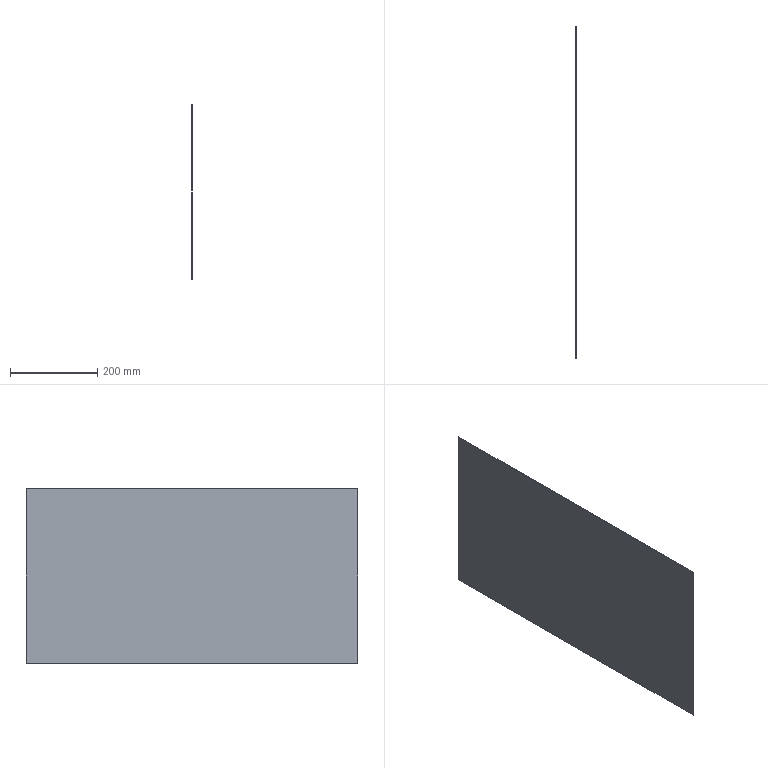Part | STEP file | Guide wheel mechanism revised.sldasm-Part-168 | 1 solid | 6 faces | box 1.2 x 760 x 400 mm | volume 364800 mm3 | plane 6
STEP:
#1=CARTESIAN_POINT('',(-360.,760.,200.));
#2=VERTEX_POINT('',#1);
#3=CARTESIAN_POINT('',(-360.,0.,200.));
#4=VERTEX_POINT('',#3);
#5=CARTESIAN_POINT('',(-360.,760.,200.));
#6=DIRECTION('',(0.,-1.,0.));
#7=VECTOR('',#6,1000.);
#8=LINE('',#5,#7);
#9=EDGE_CURVE('',#2,#4,#8,.T.);
#10=ORIENTED_EDGE('',*,*,#9,.F.);
#11=CARTESIAN_POINT('',(-361.2,760.,200.));
#12=VERTEX_POINT('',#11);
#13=CARTESIAN_POINT('',(-361.2,760.,200.));
#14=DIRECTION('',(1.,0.,0.));
#15=VECTOR('',#14,1000.);
#16=LINE('',#13,#15);
#17=EDGE_CURVE('',#12,#2,#16,.T.);
#18=ORIENTED_EDGE('',*,*,#17,.F.);
#19=CARTESIAN_POINT('',(-361.2,0.,200.));
#20=VERTEX_POINT('',#19);
#21=CARTESIAN_POINT('',(-361.2,760.,200.));
#22=DIRECTION('',(0.,-1.,0.));
#23=VECTOR('',#22,1000.);
#24=LINE('',#21,#23);
#25=EDGE_CURVE('',#12,#20,#24,.T.);
#26=ORIENTED_EDGE('',*,*,#25,.T.);
#27=CARTESIAN_POINT('',(-361.2,0.,200.));
#28=DIRECTION('',(1.,0.,0.));
#29=VECTOR('',#28,1000.);
#30=LINE('',#27,#29);
#31=EDGE_CURVE('',#20,#4,#30,.T.);
#32=ORIENTED_EDGE('',*,*,#31,.T.);
#33=EDGE_LOOP('',(#10,#18,#26,#32));
#34=FACE_OUTER_BOUND('',#33,.T.);
#35=CARTESIAN_POINT('',(-361.2,760.,200.));
#36=DIRECTION('',(0.,0.,1.));
#37=DIRECTION('',(0.,-1.,0.));
#38=AXIS2_PLACEMENT_3D('',#35,#36,#37);
#39=PLANE('',#38);
#40=ADVANCED_FACE('',(#34),#39,.T.);
#41=CARTESIAN_POINT('',(-360.,760.,-200.));
#42=VERTEX_POINT('',#41);
#43=CARTESIAN_POINT('',(-360.,760.,200.));
#44=DIRECTION('',(0.,0.,1.));
#45=VECTOR('',#44,1000.);
#46=LINE('',#43,#45);
#47=EDGE_CURVE('',#42,#2,#46,.T.);
#48=ORIENTED_EDGE('',*,*,#47,.F.);
#49=CARTESIAN_POINT('',(-361.2,760.,-200.));
#50=VERTEX_POINT('',#49);
#51=CARTESIAN_POINT('',(-361.2,760.,-200.));
#52=DIRECTION('',(1.,0.,0.));
#53=VECTOR('',#52,1000.);
#54=LINE('',#51,#53);
#55=EDGE_CURVE('',#50,#42,#54,.T.);
#56=ORIENTED_EDGE('',*,*,#55,.F.);
#57=CARTESIAN_POINT('',(-361.2,760.,200.));
#58=DIRECTION('',(0.,0.,1.));
#59=VECTOR('',#58,1000.);
#60=LINE('',#57,#59);
#61=EDGE_CURVE('',#50,#12,#60,.T.);
#62=ORIENTED_EDGE('',*,*,#61,.T.);
#63=ORIENTED_EDGE('',*,*,#17,.T.);
#64=EDGE_LOOP('',(#48,#56,#62,#63));
#65=FACE_OUTER_BOUND('',#64,.T.);
#66=CARTESIAN_POINT('',(-361.2,760.,200.));
#67=DIRECTION('',(0.,1.,0.));
#68=DIRECTION('',(0.,0.,1.));
#69=AXIS2_PLACEMENT_3D('',#66,#67,#68);
#70=PLANE('',#69);
#71=ADVANCED_FACE('',(#65),#70,.T.);
#72=CARTESIAN_POINT('',(-360.,0.,-200.));
#73=VERTEX_POINT('',#72);
#74=CARTESIAN_POINT('',(-360.,760.,-200.));
#75=DIRECTION('',(0.,1.,0.));
#76=VECTOR('',#75,1000.);
#77=LINE('',#74,#76);
#78=EDGE_CURVE('',#73,#42,#77,.T.);
#79=ORIENTED_EDGE('',*,*,#78,.F.);
#80=CARTESIAN_POINT('',(-361.2,0.,-200.));
#81=VERTEX_POINT('',#80);
#82=CARTESIAN_POINT('',(-361.2,0.,-200.));
#83=DIRECTION('',(1.,0.,0.));
#84=VECTOR('',#83,1000.);
#85=LINE('',#82,#84);
#86=EDGE_CURVE('',#81,#73,#85,.T.);
#87=ORIENTED_EDGE('',*,*,#86,.F.);
#88=CARTESIAN_POINT('',(-361.2,760.,-200.));
#89=DIRECTION('',(0.,1.,0.));
#90=VECTOR('',#89,1000.);
#91=LINE('',#88,#90);
#92=EDGE_CURVE('',#81,#50,#91,.T.);
#93=ORIENTED_EDGE('',*,*,#92,.T.);
#94=ORIENTED_EDGE('',*,*,#55,.T.);
#95=EDGE_LOOP('',(#79,#87,#93,#94));
#96=FACE_OUTER_BOUND('',#95,.T.);
#97=CARTESIAN_POINT('',(-361.2,760.,-200.));
#98=DIRECTION('',(0.,0.,-1.));
#99=DIRECTION('',(0.,1.,0.));
#100=AXIS2_PLACEMENT_3D('',#97,#98,#99);
#101=PLANE('',#100);
#102=ADVANCED_FACE('',(#96),#101,.T.);
#103=CARTESIAN_POINT('',(-360.,0.,200.));
#104=DIRECTION('',(0.,0.,-1.));
#105=VECTOR('',#104,1000.);
#106=LINE('',#103,#105);
#107=EDGE_CURVE('',#4,#73,#106,.T.);
#108=ORIENTED_EDGE('',*,*,#107,.F.);
#109=ORIENTED_EDGE('',*,*,#31,.F.);
#110=CARTESIAN_POINT('',(-361.2,0.,200.));
#111=DIRECTION('',(0.,0.,-1.));
#112=VECTOR('',#111,1000.);
#113=LINE('',#110,#112);
#114=EDGE_CURVE('',#20,#81,#113,.T.);
#115=ORIENTED_EDGE('',*,*,#114,.T.);
#116=ORIENTED_EDGE('',*,*,#86,.T.);
#117=EDGE_LOOP('',(#108,#109,#115,#116));
#118=FACE_OUTER_BOUND('',#117,.T.);
#119=CARTESIAN_POINT('',(-361.2,0.,200.));
#120=DIRECTION('',(0.,-1.,0.));
#121=DIRECTION('',(0.,0.,-1.));
#122=AXIS2_PLACEMENT_3D('',#119,#120,#121);
#123=PLANE('',#122);
#124=ADVANCED_FACE('',(#118),#123,.T.);
#125=ORIENTED_EDGE('',*,*,#25,.F.);
#126=ORIENTED_EDGE('',*,*,#61,.F.);
#127=ORIENTED_EDGE('',*,*,#92,.F.);
#128=ORIENTED_EDGE('',*,*,#114,.F.);
#129=EDGE_LOOP('',(#125,#126,#127,#128));
#130=FACE_OUTER_BOUND('',#129,.T.);
#131=CARTESIAN_POINT('',(-361.2,0.,0.));
#132=DIRECTION('',(1.,0.,0.));
#133=DIRECTION('',(0.,0.,-1.));
#134=AXIS2_PLACEMENT_3D('',#131,#132,#133);
#135=PLANE('',#134);
#136=ADVANCED_FACE('',(#130),#135,.F.);
#137=ORIENTED_EDGE('',*,*,#9,.T.);
#138=ORIENTED_EDGE('',*,*,#107,.T.);
#139=ORIENTED_EDGE('',*,*,#78,.T.);
#140=ORIENTED_EDGE('',*,*,#47,.T.);
#141=EDGE_LOOP('',(#137,#138,#139,#140));
#142=FACE_OUTER_BOUND('',#141,.T.);
#143=CARTESIAN_POINT('',(-360.,0.,0.));
#144=DIRECTION('',(1.,0.,0.));
#145=DIRECTION('',(0.,0.,-1.));
#146=AXIS2_PLACEMENT_3D('',#143,#144,#145);
#147=PLANE('',#146);
#148=ADVANCED_FACE('',(#142),#147,.T.);
#149=CLOSED_SHELL('',(#40,#71,#102,#124,#136,#148));
#150=MANIFOLD_SOLID_BREP('',#149);
#151=CARTESIAN_POINT('',(0.,0.,0.));
#152=DIRECTION('',(0.,0.,1.));
#153=DIRECTION('',(1.,0.,0.));
#154=AXIS2_PLACEMENT_3D('',#151,#152,#153);
#155=(LENGTH_UNIT()NAMED_UNIT(*)SI_UNIT(.MILLI.,.METRE.));
#156=UNCERTAINTY_MEASURE_WITH_UNIT(LENGTH_MEASURE(0.00001),#155,'','');
#157=(NAMED_UNIT(*)PLANE_ANGLE_UNIT()SI_UNIT($,.RADIAN.));
#158=(NAMED_UNIT(*)SI_UNIT($,.STERADIAN.)SOLID_ANGLE_UNIT());
#159=(GEOMETRIC_REPRESENTATION_CONTEXT(3)GLOBAL_UNCERTAINTY_ASSIGNED_CONTEXT((#156))GLOBAL_UNIT_ASSIGNED_CONTEXT((#155,#157,#158))REPRESENTATION_CONTEXT('',''));
#160=ADVANCED_BREP_SHAPE_REPRESENTATION('',(#150,#154),#159);